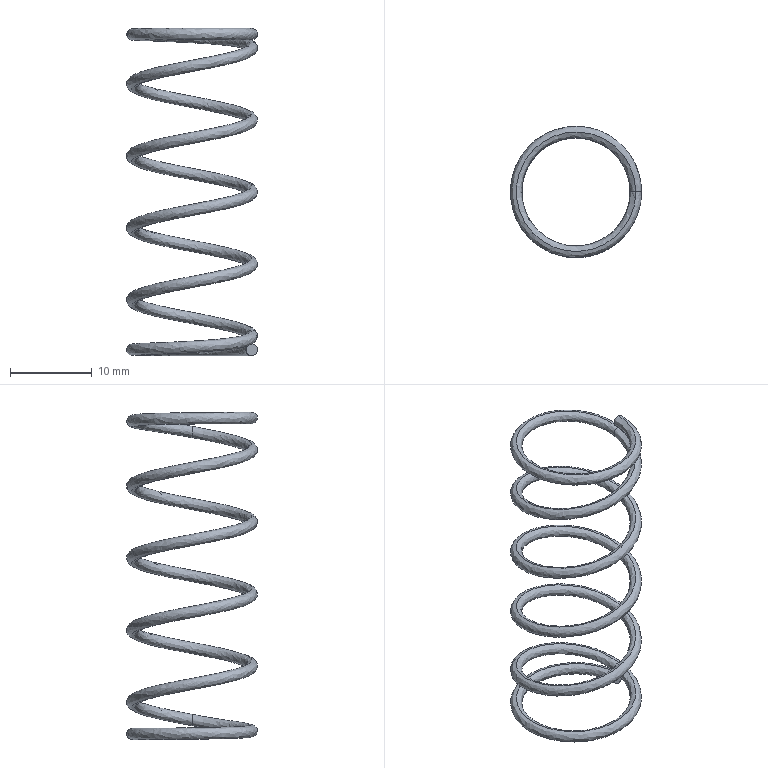Part | SolidWorks | features BaseBody 1 | 1 solid | 8 faces | box 16 x 16 x 40 mm | volume 423.431 mm3 | spline 6 | plane 2